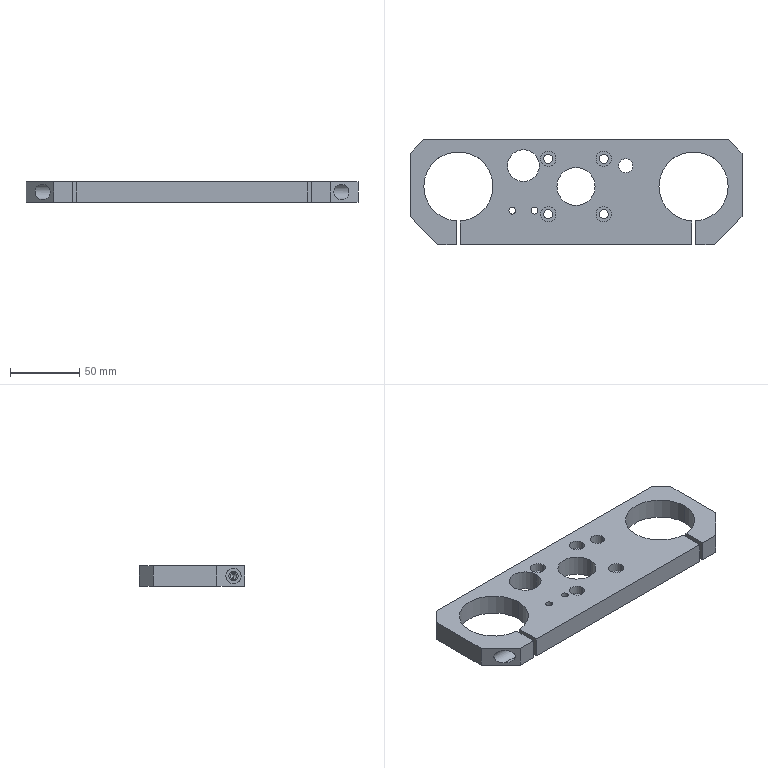Part | STEP file | PN_0048 | 1 solid | 70 faces | box 240 x 76 x 15 mm | volume 181438 mm3 | cylinder 44 | plane 22 | cone 4 | commonest cylinder face diameters 6.6 x12 11 x12 5 x8 50 x6 10.2 x2 23 x2